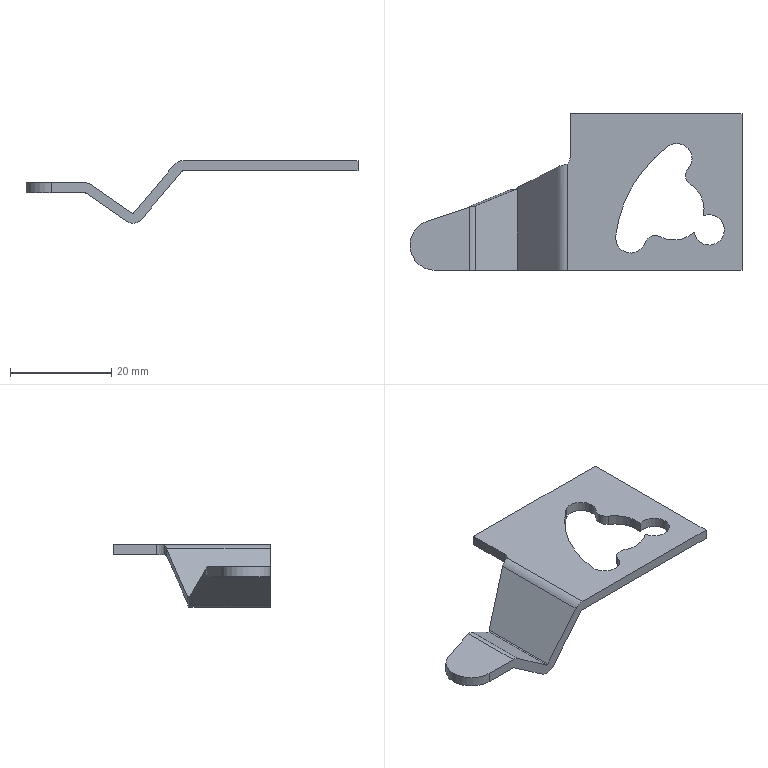Part | STEP file | door lock bent plate | 1 solid | 35 faces | box 65.681 x 31 x 12.394 mm | volume 2703 mm3 | cylinder 16 | plane 15 | spline 4 | commonest cylinder face diameters 0.6 x3 4 x3 4.6 x3 6 x3 12 x2 10 x1